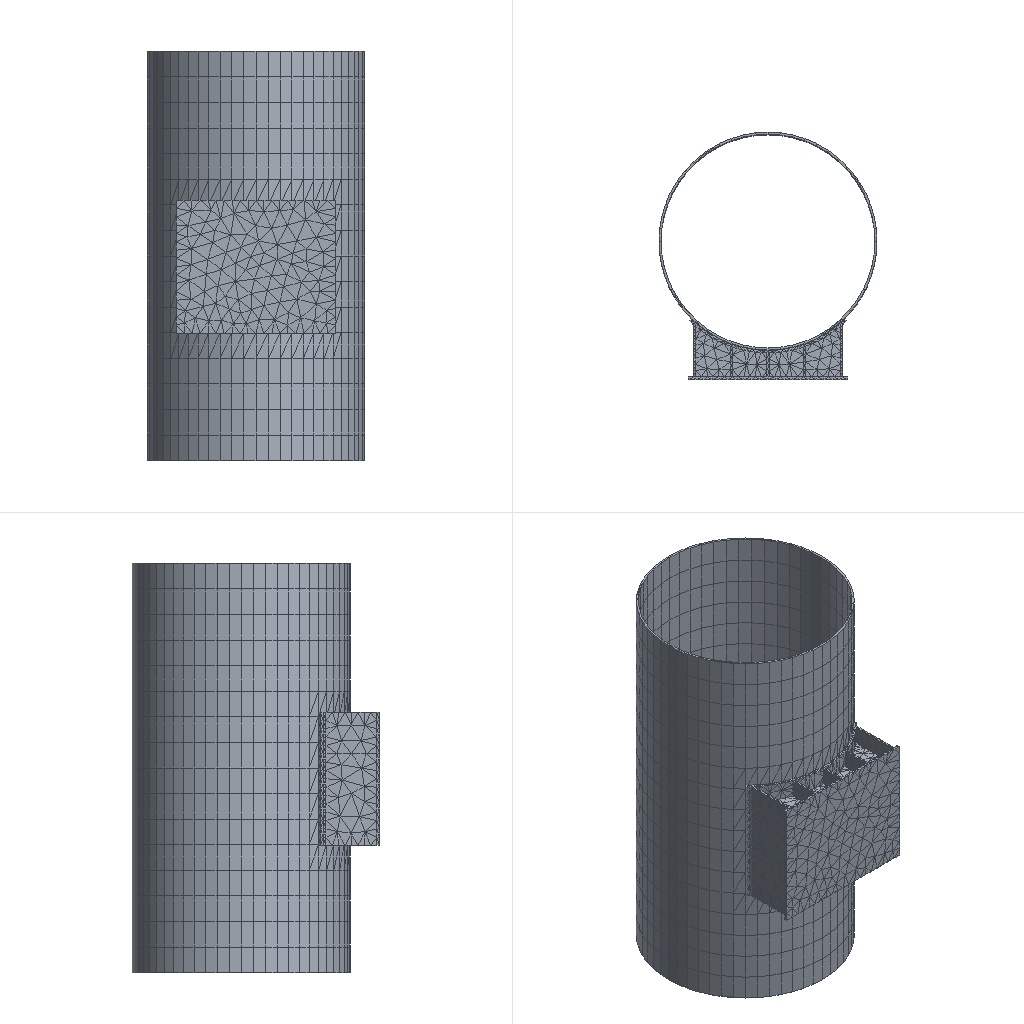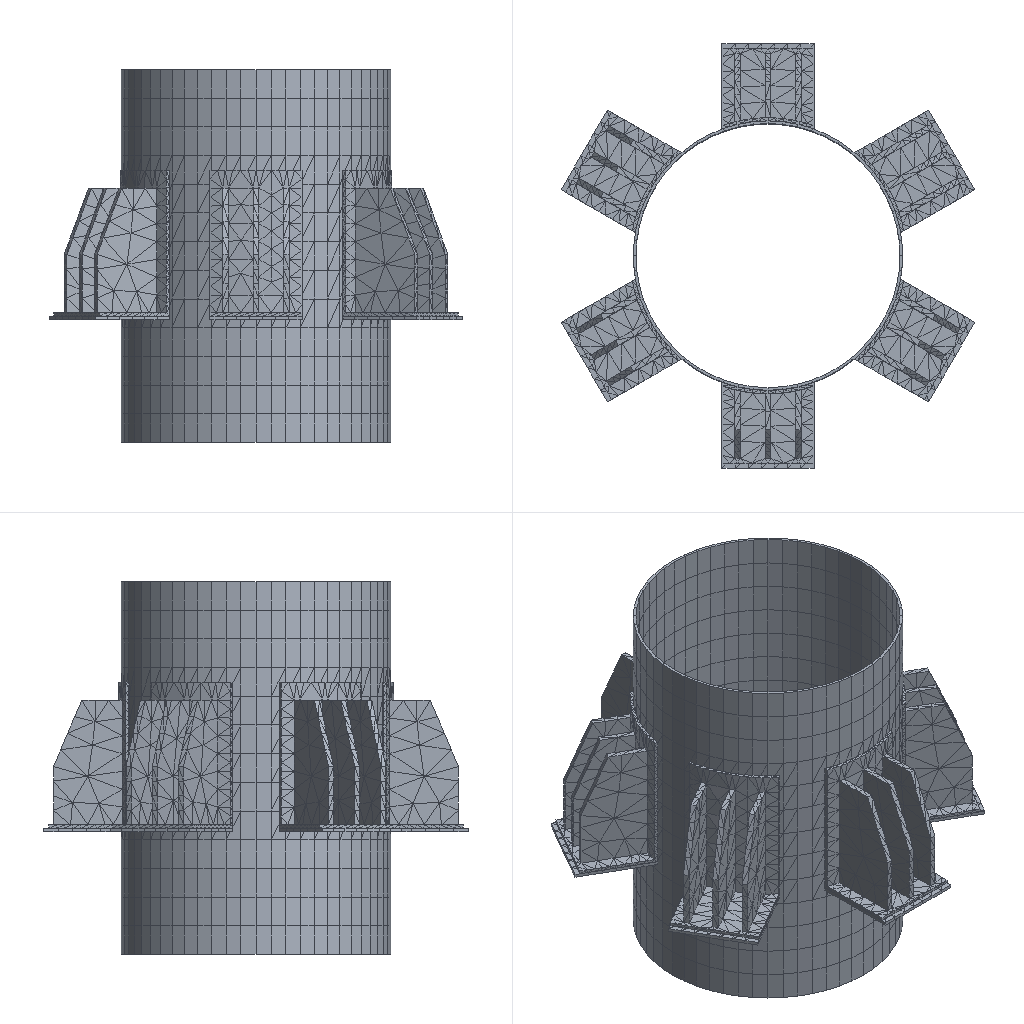Simulation study | ansys workbench
Set-up summary:
category,name,step,type,value,unit,region
solver,ansys_workbench
units,mm-N-s-tonne (MPa),,stated,"/units,MPA"
analysis,deck-1/LS1,,static
load_step,deck-1/LS1,deck-1/LS1,static,nsubst=1; time=1
analysis,deck-2/LS1,,static
load_step,deck-2/LS1,deck-2/LS1,static,nsubst=1; time=1
mesh,deck-1.dat,,nodes,17365
mesh,deck-1.dat,,elements,10691
element_type,SOLID187,,,5293,,deck-1.dat
element_type,CONTA174,,,3174,,deck-1.dat
element_type,SOLID186,,,1136,,deck-1.dat
element_type,SURF154,,,686,,deck-1.dat
element_type,TARGE170,,,402,,deck-1.dat
mesh,deck-2.dat,,nodes,20070
mesh,deck-2.dat,,elements,11206
element_type,SOLID187,,,5592,,deck-2.dat
element_type,TARGE170,,,1806,,deck-2.dat
element_type,CONTA174,,,1806,,deck-2.dat
element_type,SURF154,,,1022,,deck-2.dat
element_type,SOLID186,,,980,,deck-2.dat
material,Q345B,,E,200000,tonne s^-2 mm^-1
material,Q345B,,nu,0.3
material,Q345B,,density,7.85e-09,tonne mm^-3
material,Q345B,,conductivity,60.5,tonne mm s^-3 C^-1
material,Q345B,,specific_heat,4.34e+08,mm^2 s^-2 C^-1
material,Q345B,,cte,1.2e-05,C^-1
material,Q345B,,permeability,10000
material,Q345B,,resistivity,0.00017,ohm mm
material,Q345B,,E,200000,tonne s^-2 mm^-1
material,Q345B,,nu,0.3
material,Q345B,,density,7.85e-09,tonne mm^-3
material,Q345B,,conductivity,60.5,tonne mm s^-3 C^-1
material,Q345B,,specific_heat,4.34e+08,mm^2 s^-2 C^-1
material,Q345B,,cte,1.2e-05,C^-1
material,Q345B,,permeability,10000
material,Q345B,,resistivity,0.00017,ohm mm
load,Define Force Using Surface Effect Elements,deck-1/LS1,surface-effect pres face 2,-0.786,,SURF154 #17
load,Define Force Using Surface Effect Elements,deck-1/LS1,surface-effect pres face 1,2.615,,SURF154 #18
load,Define Force Using Surface Effect Elements,deck-1/LS1,surface-effect pres face 1,-2.615,,SURF154 #19
load,Define Force Using Surface Effect Elements,deck-1/LS1,surface-effect pres face 3,-0.985,,SURF154 #20
load,Define Force Using Surface Effect Elements,deck-1/LS1,surface-effect pres face 3,0.985,,SURF154 #21
load,,deck-1/LS1,moment,0 [n=18],,all
load,Define Force Using Surface Effect Elements,deck-2/LS1,surface-effect pres face 3,-0.6764,,SURF154 #50
load,Define Force Using Surface Effect Elements,deck-2/LS1,surface-effect pres face 1,1.12919e-14,,SURF154 #51
load,Define Force Using Surface Effect Elements,deck-2/LS1,surface-effect pres face 2,-1.613,,SURF154 #51
load,Define Force Using Surface Effect Elements,deck-2/LS1,surface-effect pres face 1,1.397,,SURF154 #52
load,Define Force Using Surface Effect Elements,deck-2/LS1,surface-effect pres face 2,-0.8066,,SURF154 #52
load,Define Force Using Surface Effect Elements,deck-2/LS1,surface-effect pres face 1,1.397,,SURF154 #53
load,Define Force Using Surface Effect Elements,deck-2/LS1,surface-effect pres face 2,0.8066,,SURF154 #53
load,Define Force Using Surface Effect Elements,deck-2/LS1,surface-effect pres face 1,1.97726e-16,,SURF154 #54
load,Define Force Using Surface Effect Elements,deck-2/LS1,surface-effect pres face 2,1.613,,SURF154 #54
load,Define Force Using Surface Effect Elements,deck-2/LS1,surface-effect pres face 1,-1.397,,SURF154 #55
load,Define Force Using Surface Effect Elements,deck-2/LS1,surface-effect pres face 2,0.8066,,SURF154 #55
bc,Fixed Supports,deck-1/model,fixed,[dofs=ALL],,_FIXEDSU
bc,Fixed Supports,deck-2/model,fixed,[dofs=ALL],,_FIXEDSU
contact,Contact Region,,bonded (always),element=CONTA174
contact,contact 2,,bonded (always),element=CONTA174
contact,contact 3,,bonded (always),element=CONTA174
contact,contact 4,,bonded (always),element=CONTA174
contact,contact 5,,bonded (always),element=CONTA174
contact,contact 6,,bonded (always),element=CONTA174
contact,contact 7,,bonded (always),element=CONTA174
contact,Contact Region,,bonded (always),element=CONTA174
contact,Contact Region 2,,bonded (always),element=CONTA174
contact,Contact Region 3,,bonded (always),element=CONTA174
contact,Contact Region 4,,bonded (always),element=CONTA174
contact,Contact Region 5,,bonded (always),element=CONTA174
contact,Contact Region 6,,bonded (always),element=CONTA174
contact,Contact Region 7,,bonded (always),element=CONTA174
contact,Contact Region 8,,bonded (always),element=CONTA174
contact,Contact Region 9,,bonded (always),element=CONTA174
contact,Contact Region 10,,bonded (always),element=CONTA174
contact,Contact Region 11,,bonded (always),element=CONTA174
contact,Contact Region 12,,bonded (always),element=CONTA174
contact,Contact Region 13,,bonded (always),element=CONTA174
contact,Contact Region 14,,bonded (always),element=CONTA174
contact,Contact Region 15,,bonded (always),element=CONTA174
contact,Contact Region 16,,bonded (always),element=CONTA174
contact,Contact Region 17,,bonded (always),element=CONTA174
contact,Contact Region 18,,bonded (always),element=CONTA174
named_set,_FIXEDSU,,node,1994
named_set,_FIXEDSU,,node,2296
Results summary:
result,analyses[0].index,,,1
result,analyses[0].system,,,SYS
result,analyses[0].deck,,,deck-1.dat
result,analyses[0].solve_status,,,completed
result,analyses[0].analysis_type,,,static
result,analyses[0].physics,,,mechanical
result,analyses[0].unit_system,,,"NMM: mm, ton, N, s, mV, mA, degC"
result,analyses[0].n_sets,,,1
result,analyses[0].load_steps[0].set,set=1,,1
result,analyses[0].load_steps[0].time_or_freq,set=1,,1
result,analyses[0].load_steps[0].max_displacement_magnitude,set=1,,0.7325
result,analyses[0].load_steps[0].max_von_mises_nodal,set=1,,209.379
result,analyses[0].load_steps[0].reaction_force_sum_xyz[1],set=1,,-0.001721
result,analyses[0].load_steps[0].reaction_force_sum_xyz[2],set=1,,1e+06
result,analyses[0].load_steps[0].reaction_force_sum_xyz[3],set=1,,0.0008563
result,analyses[1].index,,,2
result,analyses[1].system,,,SYS-1
result,analyses[1].deck,,,deck-2.dat
result,analyses[1].solve_status,,,completed
result,analyses[1].analysis_type,,,static
result,analyses[1].physics,,,mechanical
result,analyses[1].unit_system,,,"NMM: mm, ton, N, s, mV, mA, degC"
result,analyses[1].n_sets,,,1
result,analyses[1].load_steps[0].set,set=1,,1
result,analyses[1].load_steps[0].time_or_freq,set=1,,1
result,analyses[1].load_steps[0].max_displacement_magnitude,set=1,,0.215
result,analyses[1].load_steps[0].max_von_mises_nodal,set=1,,84.547
result,analyses[1].load_steps[0].reaction_force_sum_xyz[1],set=1,,-692820
result,analyses[1].load_steps[0].reaction_force_sum_xyz[2],set=1,,-400000
result,analyses[1].load_steps[0].reaction_force_sum_xyz[3],set=1,,800000